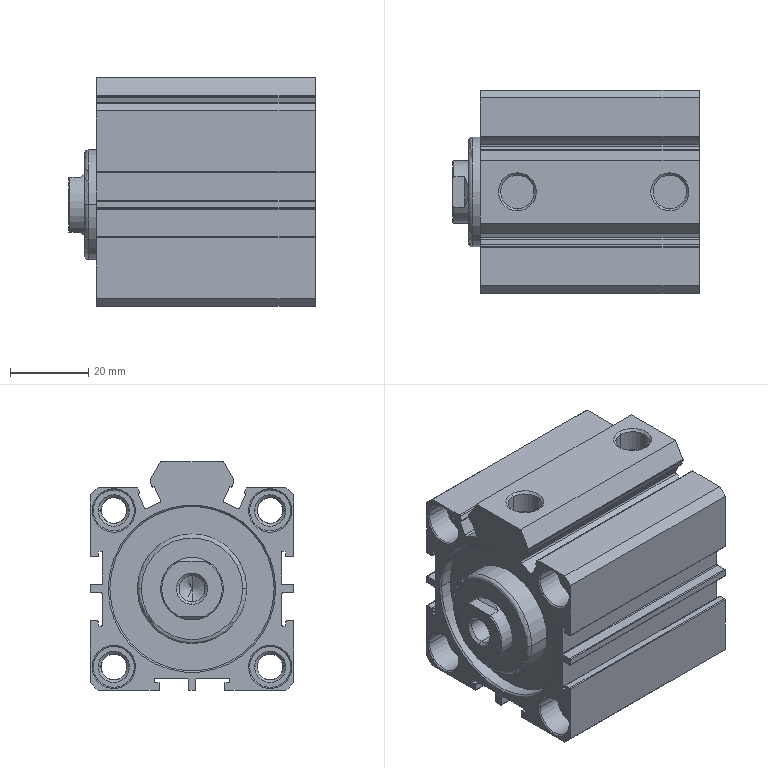Part | SolidWorks | 2 solids | 274 faces | box 63 x 52 x 58.5 mm | volume 102048 mm3 | cylinder 116 | plane 94 | cone 62 | torus 2 | commonest cylinder face diameters 0.4 x46 6.647 x18 10.5 x16 0.8 x10 6.5 x8 8.566 x4